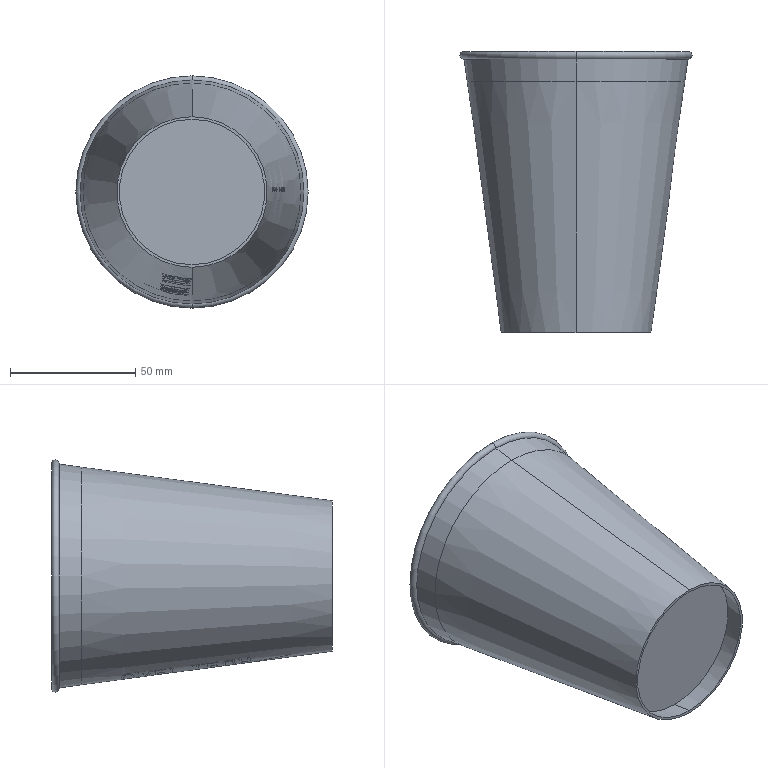Part | STEP file | Paper cup V1.201001 | 2 solids | 46 faces | box 92.598 x 112 x 92.598 mm | volume 30103 mm3 | cone 38 | plane 4 | cylinder 2 | torus 2 | commonest cylinder face diameters 60 x2